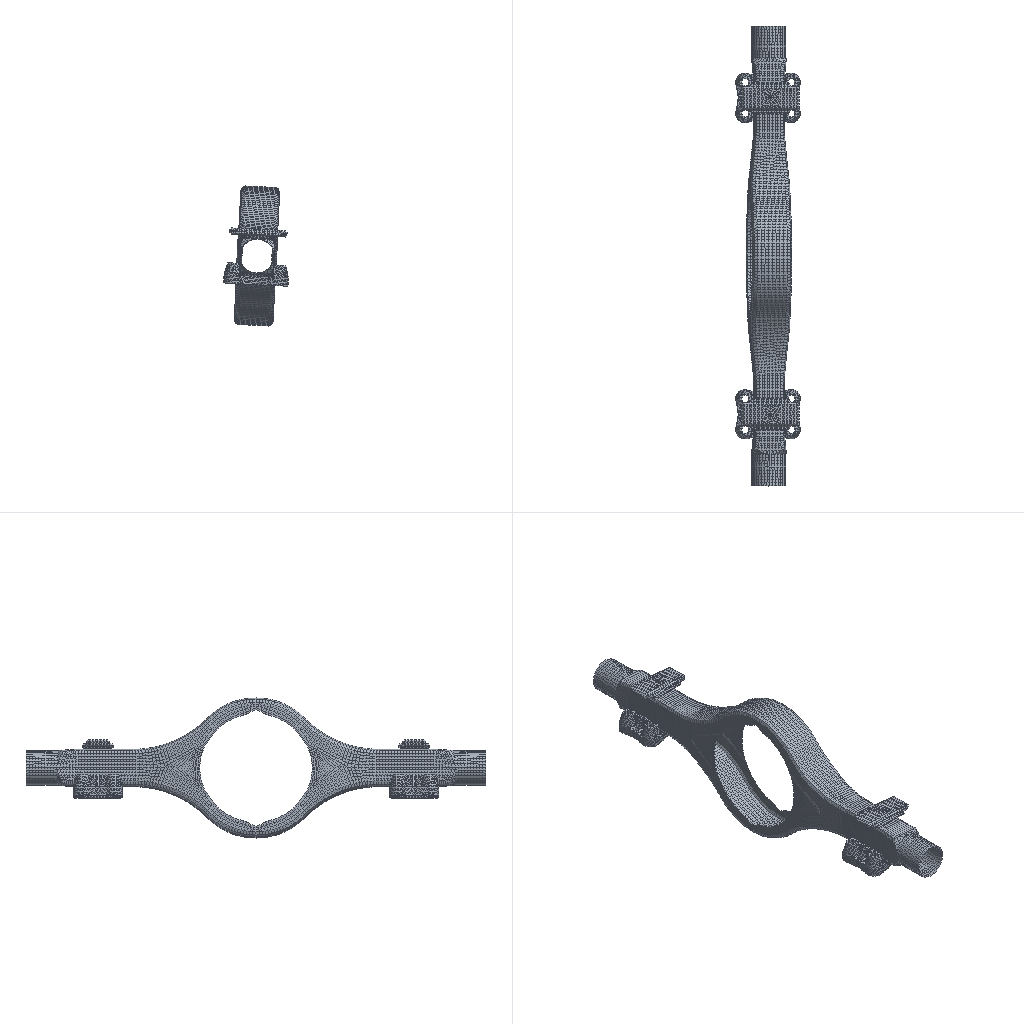Simulation study | nastran
Set-up summary:
category,name,step,type,value,unit,region
solver,nx_nastran
units,not stated in the deck,,not stated
analysis,deck,,static,static
analysis,solution,,SOL,101
load_step,SUBCASE 1,1,SUBCASE,SPC=2 LOAD=1
load_step,requested,,,1
mesh,nodes,,,12410
mesh,elements,,,23102
element_type,CQUAD4,,shell,7288
element_type,CTETRA,,solid,15746
element_type,CTRIA3,,shell,68
load,nodal force total,,FX,0.0,model units
load,nodal force total,,FY,0.0,model units
load,nodal force total,,FZ,-333200.0,model units
load,load commands in deck,,count,2
bc,support commands in deck,,count,2
check,setup vs results,,match,"every grid point's frame and coordinates and every element id; grid points of CQUAD4, CTETRA, CTRIA3 elements"
Nastran input file, long lists of numbers shortened:
$$------------------------------------------------------------------------------$
$$                                                                              $
$$ NASTRAN Input Deck Generated by HyperMesh Version  : 9.0b121                 $
$$ Generated using HyperMesh-Nastran Template Version : 9.0b121
$$                                                                              $
$$   Template:  general                                                         $
$$                                                                              $
$$------------------------------------------------------------------------------$
$$------------------------------------------------------------------------------$
$$                      Executive Control Cards                                 $
$$------------------------------------------------------------------------------$
SOL 101
CEND
$$------------------------------------------------------------------------------$
$$                      Case Control Cards                                      $
$$------------------------------------------------------------------------------$
  DISPLACEMENT(PLOT) = ALL
  STRESS(PLOT) = ALL
$
$HMNAME LOADSTEP               1"step"
SUBCASE       1
  LABEL= step
  SPC =        2
  LOAD =        1
$$------------------------------------------------------------------------------$
$$                      Bulk Data Cards                                         $
$$------------------------------------------------------------------------------$
BEGIN BULK
PARAM,POST,-1
$$
$$  GRID Data
$$
GRID         303        5238.325653.5704-439.082
GRID         304        5238.204649.8759-449.158
$ (12408 more lines like these left out)
$$
$$  SPOINT Data
$$
$$
$$------------------------------------------------------------------------------$
$$             Group Definitions                                                $
$$------------------------------------------------------------------------------$
$
$ RBE2 Elements - Single dependent node
$
RBE2       22834    5032  123456    1436
RBE2       22835    5033  123456    1468
$ (142 more lines like these left out)
$
$HMMOVE       11
$          22834THRU       22905   34453THRU       34524
$
$$
$$ RBE2 Elements - Multiple dependent nodes
$$
RBE2       34573   13825  123456    2729    3059    3121    3130    3131+
+           3132    3133    3134    3375    3376    3377    3378    3379+
+           3380    3381    3382    3383    3384    3385    3386    3387+
+           3388    3389    3434    3435    3436    3437    3438    3439+
+           3823    3824    3825    3826    3827    3828    3829    3830+
+           3831    3832    3833    3834    3835    3836    3837    4671+
+           4672    4673    4674    4675    4676    4677    4678    4679+
+           4680    4681    4682    4683    4684    4685    9853    9919+
+           9924    9928    9930    9933    9956    9958    9960    9971+
+           9974    9977    9978    9980    9990    9991    9992   10183+
+          10266   10272   10273   10276   10295   10296   10298   10299+
+          10300   10301   10302   10655   10657   10658   10659   10660+
+          10661   10662   10663   10664   10665   10666   10667   10668+
+          10669   10670   10671   11198   11199   11200   11201   11202+
+          11203   11204   11205   11206   11207   11208   11209   11210+
+          11211   11212   13800   13801   13816   13817   13818
RBE2       34574   13826  123456    2462    2515    3527    3530    3531+
+           3532    3533    3534    3550    3569    3570    3571    3572+
+           3573    3574    3575    3576    3577    3578    3579    3580+
+           3581    3582    3583    4455    4456    4457    4458    4459+
+           4460    4479    4480    4481    4482    4483    4484    4485+
+           4486    4487    4488    4489    4490    4491    4492    4493+
+           4525    4526    4527    4528    4529    4530    4531    4532+
+           4533    4534    4535    4536    4537    4538    4539    9586+
+           9639   10361   10364   10365   10366   10367   10368   10403+
+          10404   10405   10406   10407   10408   10409   10410   10411+
+          10412   10413   10414   10415   10416   10417   10982   10983+
+          10985   10986   10987   10988   10990   11036   11037   11046+
+          11048   11050   11051   11052   11056   11107   11109   11110+
+          11116   11117   11118   11119   11120   11131   11162   11165+
+          11166   11167   11168   11169   11170   11171   11172   11174+
+          11180   11185   11186   13792   13793   13808   13809
$ (168 more lines like these left out)
$
$HMMOVE       11
$          34573THRU       34582   34585   34584   34586THRU       34587
$
$$
$$  CTRIA3 Data
$$
CTRIA3       400       2     351     433     377
CTRIA3       403       2     435     440     434
$ (66 more lines like these left out)
$
$HMMOVE        7
$            400     403     409     411     615     619THRU         620     624
$       THRU         626     632     634THRU         636     643     646     648
$            654     657THRU         659     664     667     670    3295    3058
$           3046    3284    3377    3389   23022   23020   23014   23011    4319
$           4308   23226   23230THRU       23231   23235THRU       23237   23243
$          23245THRU       23247   23254   23257   23259   23265   23268THRU
$          23270   23275   23278   23281   25210   25235   25247   25501   25605
$          25617   26251   26262
$
$
$HMMOVE        8
$           4405    4578   26311   26484
$
$
$  CQUAD4 Elements
$
CQUAD4       359       2     396     373     374     410
CQUAD4       358       2     395     396     410     409
$ (7286 more lines like these left out)
$
$HMMOVE        7
$            359     358     357     356     355     354     353     352     351
$            350     349     348     347     346     345     344     343     342
$ (95 more lines like these left out)
CTETRA     26683       3   13612   13632   11354   13579
CTETRA     26682       3   13689   13215   13512   12736
$ (15744 more lines like these left out)
$
$HMMOVE        9
$          26683   26682   26681   26680   26679   26678   26677   26676   26675
$          26674   26673   26672   26671   26670   26669   26668   26667   26666
$ (665 more lines like these left out)
PSHELL         1       112.0           1               1
$
$HMNAME PROP                   2"Pshell_1400T" 4
$HWCOLOR PROP                  2      11
PSHELL         2       114.0           1               1
$$
$$  PSOLID Data
$
$HMNAME PROP                   3"solid" 5
$HWCOLOR PROP                  3      11
PSOLID         3       1
$$
$$------------------------------------------------------------------------------$
$$                      Material Definition Cards                               $
$$------------------------------------------------------------------------------$
$$--------------------------------------------------------------
$$ HYPERMESH TAGS
$$--------------------------------------------------------------
$$BEGIN TAGS
$$END TAGS
$$
$$  MAT1 Data
$
$HMNAME MAT                    1"steel" "MAT1"
$HWCOLOR MAT                   1      11
MAT1           1210000.0        0.3     7.90E-09
$$
$$
$$
$$------------------------------------------------------------------------------$
$ (37 more lines like these left out)
SPC            2   13837  1234560.0
SPC            2   13836  1234560.0
$$
$$  FORCE Data
$$
FORCE          1   13839       01.0     0.0     0.0     -166600.
FORCE          1   13838       01.0     0.0     0.0     -166600.
$
ENDDATA
Results summary:
result,analysis,,,static
result,last_loadstep,,,1
result,primary field,,,displacements
result,max displacement,,,0.3392,model units